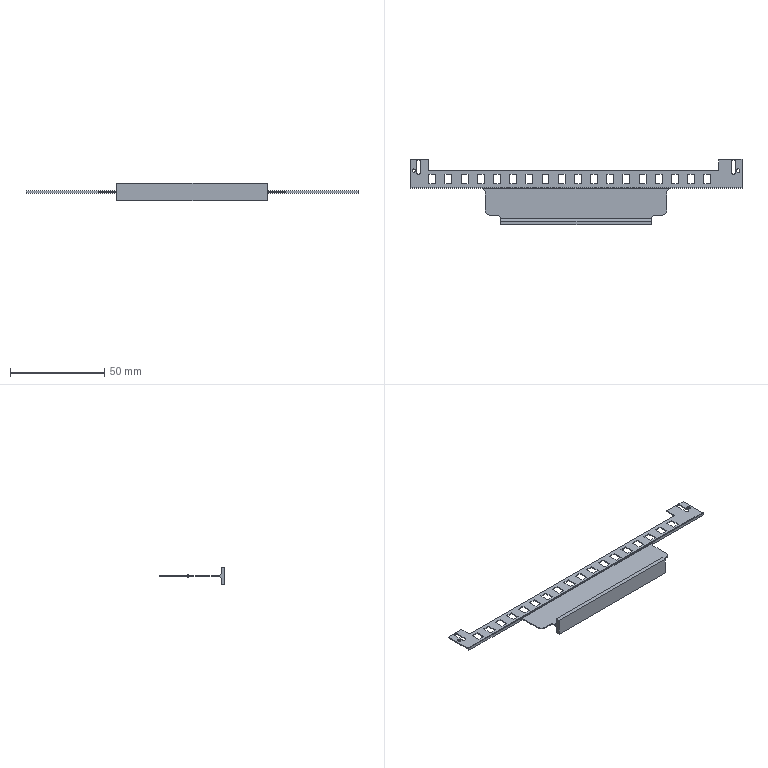Part | SolidWorks | features ICE 13, Fillet 3, Cut 1, Extrusion 1 | 1 solid | 121 faces | box 176.5 x 35 x 9.08 mm | volume 3160 mm3 | plane 105 | cylinder 16 | commonest cylinder face diameters 2 x4 6 x4 1.757 x2 1.874 x2 3 x2 4 x2